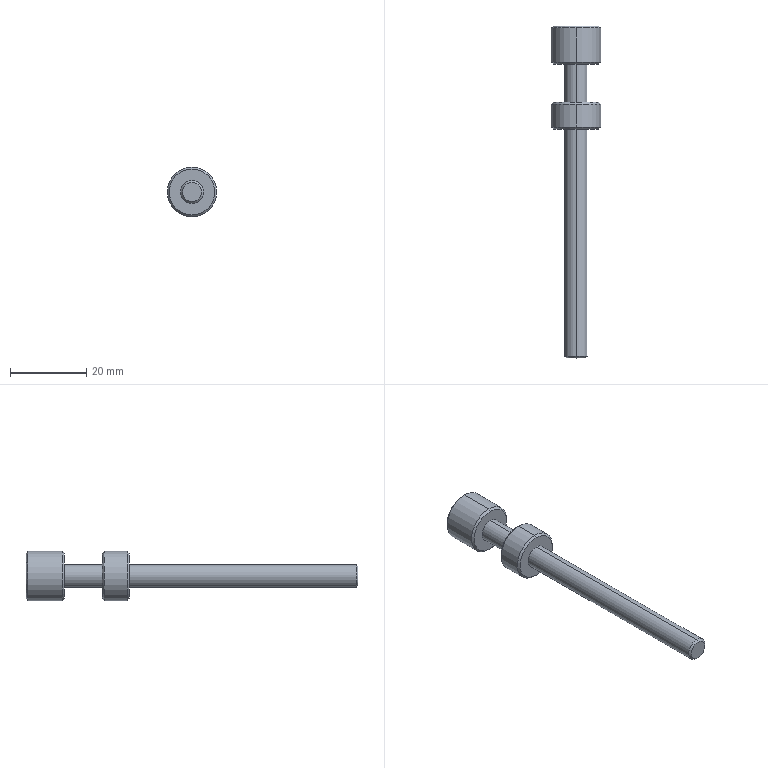Part | SolidWorks | features ICE 5, Chamfer 1, Extrusion 1 | 1 solid | 30 faces | box 13 x 87 x 13 mm | volume 4026 mm3 | plane 12 | cone 10 | cylinder 8 | commonest cylinder face diameters 6 x4 13 x4
STEP:
#1=CARTESIAN_POINT('',(0.,67.,6.));
#2=VERTEX_POINT('',#1);
#3=CARTESIAN_POINT('',(0.,67.,-6.));
#4=VERTEX_POINT('',#3);
#5=CARTESIAN_POINT('',(0.,67.,0.));
#6=DIRECTION('',(0.,1.,0.));
#7=DIRECTION('',(0.,0.,1.));
#8=AXIS2_PLACEMENT_3D('',#5,#6,#7);
#9=CIRCLE('',#8,6.);
#10=EDGE_CURVE('',#2,#4,#9,.T.);
#11=ORIENTED_EDGE('',*,*,#10,.F.);
#12=CARTESIAN_POINT('',(0.,66.5,6.5));
#13=VERTEX_POINT('',#12);
#14=CARTESIAN_POINT('',(0.,67.,6.));
#15=DIRECTION('',(0.,-0.7071,0.7071));
#16=VECTOR('',#15,1000.);
#17=LINE('',#14,#16);
#18=EDGE_CURVE('',#2,#13,#17,.T.);
#19=ORIENTED_EDGE('',*,*,#18,.T.);
#20=CARTESIAN_POINT('',(0.,66.5,-6.5));
#21=VERTEX_POINT('',#20);
#22=CARTESIAN_POINT('',(0.,66.5,0.));
#23=DIRECTION('',(0.,-1.,0.));
#24=DIRECTION('',(0.,0.,1.));
#25=AXIS2_PLACEMENT_3D('',#22,#23,#24);
#26=CIRCLE('',#25,6.5);
#27=EDGE_CURVE('',#21,#13,#26,.T.);
#28=ORIENTED_EDGE('',*,*,#27,.F.);
#29=CARTESIAN_POINT('',(0.,67.,-6.));
#30=DIRECTION('',(0.,-0.7071,-0.7071));
#31=VECTOR('',#30,1000.);
#32=LINE('',#29,#31);
#33=EDGE_CURVE('',#4,#21,#32,.T.);
#34=ORIENTED_EDGE('',*,*,#33,.F.);
#35=EDGE_LOOP('',(#11,#19,#28,#34));
#36=FACE_OUTER_BOUND('',#35,.T.);
#37=CARTESIAN_POINT('',(0.,67.,0.));
#38=DIRECTION('',(0.,-1.,0.));
#39=DIRECTION('',(0.,0.,-1.));
#40=AXIS2_PLACEMENT_3D('',#37,#38,#39);
#41=CONICAL_SURFACE('',#40,6.,0.7854);
#42=ADVANCED_FACE('',(#36),#41,.T.);
#43=CARTESIAN_POINT('',(0.,60.,-6.));
#44=VERTEX_POINT('',#43);
#45=CARTESIAN_POINT('',(0.,60.,6.));
#46=VERTEX_POINT('',#45);
#47=CARTESIAN_POINT('',(0.,60.,0.));
#48=DIRECTION('',(0.,-1.,0.));
#49=DIRECTION('',(0.,0.,1.));
#50=AXIS2_PLACEMENT_3D('',#47,#48,#49);
#51=CIRCLE('',#50,6.);
#52=EDGE_CURVE('',#44,#46,#51,.T.);
#53=ORIENTED_EDGE('',*,*,#52,.F.);
#54=CARTESIAN_POINT('',(0.,60.5,-6.5));
#55=VERTEX_POINT('',#54);
#56=CARTESIAN_POINT('',(0.,60.5,-6.5));
#57=DIRECTION('',(0.,0.7071,-0.7071));
#58=VECTOR('',#57,1000.);
#59=LINE('',#56,#58);
#60=EDGE_CURVE('',#44,#55,#59,.T.);
#61=ORIENTED_EDGE('',*,*,#60,.T.);
#62=CARTESIAN_POINT('',(0.,60.5,6.5));
#63=VERTEX_POINT('',#62);
#64=CARTESIAN_POINT('',(0.,60.5,0.));
#65=DIRECTION('',(0.,1.,0.));
#66=DIRECTION('',(0.,0.,1.));
#67=AXIS2_PLACEMENT_3D('',#64,#65,#66);
#68=CIRCLE('',#67,6.5);
#69=EDGE_CURVE('',#63,#55,#68,.T.);
#70=ORIENTED_EDGE('',*,*,#69,.F.);
#71=CARTESIAN_POINT('',(0.,60.5,6.5));
#72=DIRECTION('',(0.,0.7071,0.7071));
#73=VECTOR('',#72,1000.);
#74=LINE('',#71,#73);
#75=EDGE_CURVE('',#46,#63,#74,.T.);
#76=ORIENTED_EDGE('',*,*,#75,.F.);
#77=EDGE_LOOP('',(#53,#61,#70,#76));
#78=FACE_OUTER_BOUND('',#77,.T.);
#79=CARTESIAN_POINT('',(0.,60.5,0.));
#80=DIRECTION('',(0.,1.,0.));
#81=DIRECTION('',(0.,0.,1.));
#82=AXIS2_PLACEMENT_3D('',#79,#80,#81);
#83=CONICAL_SURFACE('',#82,6.5,0.7854);
#84=ADVANCED_FACE('',(#78),#83,.T.);
#85=CARTESIAN_POINT('',(0.,77.,-6.));
#86=VERTEX_POINT('',#85);
#87=CARTESIAN_POINT('',(0.,77.,6.));
#88=VERTEX_POINT('',#87);
#89=CARTESIAN_POINT('',(0.,77.,0.));
#90=DIRECTION('',(0.,-1.,0.));
#91=DIRECTION('',(0.,0.,1.));
#92=AXIS2_PLACEMENT_3D('',#89,#90,#91);
#93=CIRCLE('',#92,6.);
#94=EDGE_CURVE('',#86,#88,#93,.T.);
#95=ORIENTED_EDGE('',*,*,#94,.F.);
#96=CARTESIAN_POINT('',(0.,77.5,-6.5));
#97=VERTEX_POINT('',#96);
#98=CARTESIAN_POINT('',(0.,77.5,-6.5));
#99=DIRECTION('',(0.,0.7071,-0.7071));
#100=VECTOR('',#99,1000.);
#101=LINE('',#98,#100);
#102=EDGE_CURVE('',#86,#97,#101,.T.);
#103=ORIENTED_EDGE('',*,*,#102,.T.);
#104=CARTESIAN_POINT('',(0.,77.5,6.5));
#105=VERTEX_POINT('',#104);
#106=CARTESIAN_POINT('',(0.,77.5,0.));
#107=DIRECTION('',(0.,1.,0.));
#108=DIRECTION('',(0.,0.,1.));
#109=AXIS2_PLACEMENT_3D('',#106,#107,#108);
#110=CIRCLE('',#109,6.5);
#111=EDGE_CURVE('',#105,#97,#110,.T.);
#112=ORIENTED_EDGE('',*,*,#111,.F.);
#113=CARTESIAN_POINT('',(0.,77.5,6.5));
#114=DIRECTION('',(0.,0.7071,0.7071));
#115=VECTOR('',#114,1000.);
#116=LINE('',#113,#115);
#117=EDGE_CURVE('',#88,#105,#116,.T.);
#118=ORIENTED_EDGE('',*,*,#117,.F.);
#119=EDGE_LOOP('',(#95,#103,#112,#118));
#120=FACE_OUTER_BOUND('',#119,.T.);
#121=CARTESIAN_POINT('',(0.,77.5,0.));
#122=DIRECTION('',(0.,1.,0.));
#123=DIRECTION('',(0.,0.,1.));
#124=AXIS2_PLACEMENT_3D('',#121,#122,#123);
#125=CONICAL_SURFACE('',#124,6.5,0.7854);
#126=ADVANCED_FACE('',(#120),#125,.T.);
#127=CARTESIAN_POINT('',(0.,87.,6.));
#128=VERTEX_POINT('',#127);
#129=CARTESIAN_POINT('',(0.,87.,-6.));
#130=VERTEX_POINT('',#129);
#131=CARTESIAN_POINT('',(0.,87.,0.));
#132=DIRECTION('',(0.,1.,0.));
#133=DIRECTION('',(0.,0.,1.));
#134=AXIS2_PLACEMENT_3D('',#131,#132,#133);
#135=CIRCLE('',#134,6.);
#136=EDGE_CURVE('',#128,#130,#135,.T.);
#137=ORIENTED_EDGE('',*,*,#136,.F.);
#138=CARTESIAN_POINT('',(0.,86.5,6.5));
#139=VERTEX_POINT('',#138);
#140=CARTESIAN_POINT('',(0.,87.,6.));
#141=DIRECTION('',(0.,-0.7071,0.7071));
#142=VECTOR('',#141,1000.);
#143=LINE('',#140,#142);
#144=EDGE_CURVE('',#128,#139,#143,.T.);
#145=ORIENTED_EDGE('',*,*,#144,.T.);
#146=CARTESIAN_POINT('',(0.,86.5,-6.5));
#147=VERTEX_POINT('',#146);
#148=CARTESIAN_POINT('',(0.,86.5,0.));
#149=DIRECTION('',(0.,-1.,0.));
#150=DIRECTION('',(0.,0.,1.));
#151=AXIS2_PLACEMENT_3D('',#148,#149,#150);
#152=CIRCLE('',#151,6.5);
#153=EDGE_CURVE('',#147,#139,#152,.T.);
#154=ORIENTED_EDGE('',*,*,#153,.F.);
#155=CARTESIAN_POINT('',(0.,87.,-6.));
#156=DIRECTION('',(0.,-0.7071,-0.7071));
#157=VECTOR('',#156,1000.);
#158=LINE('',#155,#157);
#159=EDGE_CURVE('',#130,#147,#158,.T.);
#160=ORIENTED_EDGE('',*,*,#159,.F.);
#161=EDGE_LOOP('',(#137,#145,#154,#160));
#162=FACE_OUTER_BOUND('',#161,.T.);
#163=CARTESIAN_POINT('',(0.,87.,0.));
#164=DIRECTION('',(0.,-1.,0.));
#165=DIRECTION('',(0.,0.,-1.));
#166=AXIS2_PLACEMENT_3D('',#163,#164,#165);
#167=CONICAL_SURFACE('',#166,6.,0.7854);
#168=ADVANCED_FACE('',(#162),#167,.T.);
#169=CARTESIAN_POINT('',(0.,0.,-2.5));
#170=VERTEX_POINT('',#169);
#171=CARTESIAN_POINT('',(0.,0.,2.5));
#172=VERTEX_POINT('',#171);
#173=CARTESIAN_POINT('',(0.,0.,0.));
#174=DIRECTION('',(0.,-1.,0.));
#175=DIRECTION('',(0.,0.,1.));
#176=AXIS2_PLACEMENT_3D('',#173,#174,#175);
#177=CIRCLE('',#176,2.5);
#178=EDGE_CURVE('',#170,#172,#177,.T.);
#179=ORIENTED_EDGE('',*,*,#178,.F.);
#180=CARTESIAN_POINT('',(0.,0.5,-3.));
#181=VERTEX_POINT('',#180);
#182=CARTESIAN_POINT('',(0.,0.5,-3.));
#183=DIRECTION('',(0.,0.7071,-0.7071));
#184=VECTOR('',#183,1000.);
#185=LINE('',#182,#184);
#186=EDGE_CURVE('',#170,#181,#185,.T.);
#187=ORIENTED_EDGE('',*,*,#186,.T.);
#188=CARTESIAN_POINT('',(0.,0.5,3.));
#189=VERTEX_POINT('',#188);
#190=CARTESIAN_POINT('',(0.,0.5,0.));
#191=DIRECTION('',(0.,1.,0.));
#192=DIRECTION('',(0.,0.,1.));
#193=AXIS2_PLACEMENT_3D('',#190,#191,#192);
#194=CIRCLE('',#193,3.);
#195=EDGE_CURVE('',#189,#181,#194,.T.);
#196=ORIENTED_EDGE('',*,*,#195,.F.);
#197=CARTESIAN_POINT('',(0.,0.5,3.));
#198=DIRECTION('',(0.,0.7071,0.7071));
#199=VECTOR('',#198,1000.);
#200=LINE('',#197,#199);
#201=EDGE_CURVE('',#172,#189,#200,.T.);
#202=ORIENTED_EDGE('',*,*,#201,.F.);
#203=EDGE_LOOP('',(#179,#187,#196,#202));
#204=FACE_OUTER_BOUND('',#203,.T.);
#205=CARTESIAN_POINT('',(0.,0.5,0.));
#206=DIRECTION('',(0.,1.,0.));
#207=DIRECTION('',(0.,0.,1.));
#208=AXIS2_PLACEMENT_3D('',#205,#206,#207);
#209=CONICAL_SURFACE('',#208,3.,0.7854);
#210=ADVANCED_FACE('',(#204),#209,.T.);
#211=ORIENTED_EDGE('',*,*,#153,.T.);
#212=CARTESIAN_POINT('',(0.,87.,6.5));
#213=DIRECTION('',(0.,-1.,0.));
#214=VECTOR('',#213,1000.);
#215=LINE('',#212,#214);
#216=EDGE_CURVE('',#139,#105,#215,.T.);
#217=ORIENTED_EDGE('',*,*,#216,.T.);
#218=ORIENTED_EDGE('',*,*,#111,.T.);
#219=CARTESIAN_POINT('',(0.,87.,-6.5));
#220=DIRECTION('',(0.,-1.,0.));
#221=VECTOR('',#220,1000.);
#222=LINE('',#219,#221);
#223=EDGE_CURVE('',#147,#97,#222,.T.);
#224=ORIENTED_EDGE('',*,*,#223,.F.);
#225=EDGE_LOOP('',(#211,#217,#218,#224));
#226=FACE_OUTER_BOUND('',#225,.T.);
#227=CARTESIAN_POINT('',(0.,87.,0.));
#228=DIRECTION('',(0.,-1.,0.));
#229=DIRECTION('',(0.,0.,-1.));
#230=AXIS2_PLACEMENT_3D('',#227,#228,#229);
#231=CYLINDRICAL_SURFACE('',#230,6.5);
#232=ADVANCED_FACE('',(#226),#231,.T.);
#233=CARTESIAN_POINT('',(0.,77.,3.));
#234=VERTEX_POINT('',#233);
#235=CARTESIAN_POINT('',(0.,77.,-3.));
#236=VERTEX_POINT('',#235);
#237=CARTESIAN_POINT('',(0.,77.,0.));
#238=DIRECTION('',(0.,1.,0.));
#239=DIRECTION('',(0.,0.,1.));
#240=AXIS2_PLACEMENT_3D('',#237,#238,#239);
#241=CIRCLE('',#240,3.);
#242=EDGE_CURVE('',#234,#236,#241,.T.);
#243=ORIENTED_EDGE('',*,*,#242,.F.);
#244=CARTESIAN_POINT('',(0.,67.,3.));
#245=VERTEX_POINT('',#244);
#246=CARTESIAN_POINT('',(0.,77.,3.));
#247=DIRECTION('',(0.,-1.,0.));
#248=VECTOR('',#247,1000.);
#249=LINE('',#246,#248);
#250=EDGE_CURVE('',#234,#245,#249,.T.);
#251=ORIENTED_EDGE('',*,*,#250,.T.);
#252=CARTESIAN_POINT('',(0.,67.,-3.));
#253=VERTEX_POINT('',#252);
#254=CARTESIAN_POINT('',(0.,67.,0.));
#255=DIRECTION('',(0.,1.,0.));
#256=DIRECTION('',(0.,0.,1.));
#257=AXIS2_PLACEMENT_3D('',#254,#255,#256);
#258=CIRCLE('',#257,3.);
#259=EDGE_CURVE('',#245,#253,#258,.T.);
#260=ORIENTED_EDGE('',*,*,#259,.T.);
#261=CARTESIAN_POINT('',(0.,77.,-3.));
#262=DIRECTION('',(0.,-1.,0.));
#263=VECTOR('',#262,1000.);
#264=LINE('',#261,#263);
#265=EDGE_CURVE('',#236,#253,#264,.T.);
#266=ORIENTED_EDGE('',*,*,#265,.F.);
#267=EDGE_LOOP('',(#243,#251,#260,#266));
#268=FACE_OUTER_BOUND('',#267,.T.);
#269=CARTESIAN_POINT('',(0.,77.,0.));
#270=DIRECTION('',(0.,-1.,0.));
#271=DIRECTION('',(0.,0.,-1.));
#272=AXIS2_PLACEMENT_3D('',#269,#270,#271);
#273=CYLINDRICAL_SURFACE('',#272,3.);
#274=ADVANCED_FACE('',(#268),#273,.T.);
#275=ORIENTED_EDGE('',*,*,#27,.T.);
#276=CARTESIAN_POINT('',(0.,67.,6.5));
#277=DIRECTION('',(0.,-1.,0.));
#278=VECTOR('',#277,1000.);
#279=LINE('',#276,#278);
#280=EDGE_CURVE('',#13,#63,#279,.T.);
#281=ORIENTED_EDGE('',*,*,#280,.T.);
#282=ORIENTED_EDGE('',*,*,#69,.T.);
#283=CARTESIAN_POINT('',(0.,67.,-6.5));
#284=DIRECTION('',(0.,-1.,0.));
#285=VECTOR('',#284,1000.);
#286=LINE('',#283,#285);
#287=EDGE_CURVE('',#21,#55,#286,.T.);
#288=ORIENTED_EDGE('',*,*,#287,.F.);
#289=EDGE_LOOP('',(#275,#281,#282,#288));
#290=FACE_OUTER_BOUND('',#289,.T.);
#291=CARTESIAN_POINT('',(0.,67.,0.));
#292=DIRECTION('',(0.,-1.,0.));
#293=DIRECTION('',(0.,0.,-1.));
#294=AXIS2_PLACEMENT_3D('',#291,#292,#293);
#295=CYLINDRICAL_SURFACE('',#294,6.5);
#296=ADVANCED_FACE('',(#290),#295,.T.);
#297=CARTESIAN_POINT('',(0.,60.,3.));
#298=VERTEX_POINT('',#297);
#299=CARTESIAN_POINT('',(0.,60.,-3.));
#300=VERTEX_POINT('',#299);
#301=CARTESIAN_POINT('',(0.,60.,0.));
#302=DIRECTION('',(0.,1.,0.));
#303=DIRECTION('',(0.,0.,1.));
#304=AXIS2_PLACEMENT_3D('',#301,#302,#303);
#305=CIRCLE('',#304,3.);
#306=EDGE_CURVE('',#298,#300,#305,.T.);
#307=ORIENTED_EDGE('',*,*,#306,.F.);
#308=CARTESIAN_POINT('',(0.,45.,3.));
#309=DIRECTION('',(0.,-1.,0.));
#310=VECTOR('',#309,1000.);
#311=LINE('',#308,#310);
#312=EDGE_CURVE('',#298,#189,#311,.T.);
#313=ORIENTED_EDGE('',*,*,#312,.T.);
#314=ORIENTED_EDGE('',*,*,#195,.T.);
#315=CARTESIAN_POINT('',(0.,45.,-3.));
#316=DIRECTION('',(0.,-1.,0.));
#317=VECTOR('',#316,1000.);
#318=LINE('',#315,#317);
#319=EDGE_CURVE('',#300,#181,#318,.T.);
#320=ORIENTED_EDGE('',*,*,#319,.F.);
#321=EDGE_LOOP('',(#307,#313,#314,#320));
#322=FACE_OUTER_BOUND('',#321,.T.);
#323=CARTESIAN_POINT('',(0.,45.,0.));
#324=DIRECTION('',(0.,-1.,0.));
#325=DIRECTION('',(0.,0.,-1.));
#326=AXIS2_PLACEMENT_3D('',#323,#324,#325);
#327=CYLINDRICAL_SURFACE('',#326,3.);
#328=ADVANCED_FACE('',(#322),#327,.T.);
#329=CARTESIAN_POINT('',(0.,67.,0.));
#330=DIRECTION('',(0.,1.,0.));
#331=DIRECTION('',(0.,0.,1.));
#332=AXIS2_PLACEMENT_3D('',#329,#330,#331);
#333=CIRCLE('',#332,6.);
#334=EDGE_CURVE('',#4,#2,#333,.T.);
#335=ORIENTED_EDGE('',*,*,#334,.T.);
#336=ORIENTED_EDGE('',*,*,#10,.T.);
#337=EDGE_LOOP('',(#335,#336));
#338=FACE_OUTER_BOUND('',#337,.T.);
#339=CARTESIAN_POINT('',(0.,67.,0.));
#340=DIRECTION('',(0.,1.,0.));
#341=DIRECTION('',(0.,0.,1.));
#342=AXIS2_PLACEMENT_3D('',#339,#340,#341);
#343=CIRCLE('',#342,3.);
#344=EDGE_CURVE('',#253,#245,#343,.T.);
#345=ORIENTED_EDGE('',*,*,#344,.F.);
#346=ORIENTED_EDGE('',*,*,#259,.F.);
#347=EDGE_LOOP('',(#345,#346));
#348=FACE_BOUND('',#347,.T.);
#349=CARTESIAN_POINT('',(0.,67.,0.));
#350=DIRECTION('',(0.,1.,0.));
#351=DIRECTION('',(0.,0.,1.));
#352=AXIS2_PLACEMENT_3D('',#349,#350,#351);
#353=PLANE('',#352);
#354=ADVANCED_FACE('',(#338,#348),#353,.T.);
#355=ORIENTED_EDGE('',*,*,#312,.F.);
#356=CARTESIAN_POINT('',(0.,60.,0.));
#357=DIRECTION('',(0.,1.,0.));
#358=DIRECTION('',(0.,0.,1.));
#359=AXIS2_PLACEMENT_3D('',#356,#357,#358);
#360=CIRCLE('',#359,3.);
#361=EDGE_CURVE('',#300,#298,#360,.T.);
#362=ORIENTED_EDGE('',*,*,#361,.F.);
#363=ORIENTED_EDGE('',*,*,#319,.T.);
#364=CARTESIAN_POINT('',(0.,0.5,0.));
#365=DIRECTION('',(0.,1.,0.));
#366=DIRECTION('',(0.,0.,1.));
#367=AXIS2_PLACEMENT_3D('',#364,#365,#366);
#368=CIRCLE('',#367,3.);
#369=EDGE_CURVE('',#181,#189,#368,.T.);
#370=ORIENTED_EDGE('',*,*,#369,.T.);
#371=EDGE_LOOP('',(#355,#362,#363,#370));
#372=FACE_OUTER_BOUND('',#371,.T.);
#373=CARTESIAN_POINT('',(0.,45.,0.));
#374=DIRECTION('',(0.,-1.,0.));
#375=DIRECTION('',(0.,0.,-1.));
#376=AXIS2_PLACEMENT_3D('',#373,#374,#375);
#377=CYLINDRICAL_SURFACE('',#376,3.);
#378=ADVANCED_FACE('',(#372),#377,.T.);
#379=CARTESIAN_POINT('',(0.,0.,0.));
#380=DIRECTION('',(0.,-1.,0.));
#381=DIRECTION('',(0.,0.,1.));
#382=AXIS2_PLACEMENT_3D('',#379,#380,#381);
#383=CIRCLE('',#382,2.5);
#384=EDGE_CURVE('',#172,#170,#383,.T.);
#385=ORIENTED_EDGE('',*,*,#384,.T.);
#386=ORIENTED_EDGE('',*,*,#178,.T.);
#387=EDGE_LOOP('',(#385,#386));
#388=FACE_OUTER_BOUND('',#387,.T.);
#389=CARTESIAN_POINT('',(0.,0.,0.));
#390=DIRECTION('',(0.,1.,0.));
#391=DIRECTION('',(0.,0.,1.));
#392=AXIS2_PLACEMENT_3D('',#389,#390,#391);
#393=PLANE('',#392);
#394=ADVANCED_FACE('',(#388),#393,.F.);
#395=CARTESIAN_POINT('',(0.,60.,0.));
#396=DIRECTION('',(0.,-1.,0.));
#397=DIRECTION('',(0.,0.,1.));
#398=AXIS2_PLACEMENT_3D('',#395,#396,#397);
#399=CIRCLE('',#398,6.);
#400=EDGE_CURVE('',#46,#44,#399,.T.);
#401=ORIENTED_EDGE('',*,*,#400,.T.);
#402=ORIENTED_EDGE('',*,*,#52,.T.);
#403=EDGE_LOOP('',(#401,#402));
#404=FACE_OUTER_BOUND('',#403,.T.);
#405=ORIENTED_EDGE('',*,*,#361,.T.);
#406=ORIENTED_EDGE('',*,*,#306,.T.);
#407=EDGE_LOOP('',(#405,#406));
#408=FACE_BOUND('',#407,.T.);
#409=CARTESIAN_POINT('',(0.,60.,0.));
#410=DIRECTION('',(0.,1.,0.));
#411=DIRECTION('',(0.,0.,1.));
#412=AXIS2_PLACEMENT_3D('',#409,#410,#411);
#413=PLANE('',#412);
#414=ADVANCED_FACE('',(#404,#408),#413,.F.);
#415=ORIENTED_EDGE('',*,*,#280,.F.);
#416=CARTESIAN_POINT('',(0.,66.5,0.));
#417=DIRECTION('',(0.,-1.,0.));
#418=DIRECTION('',(0.,0.,1.));
#419=AXIS2_PLACEMENT_3D('',#416,#417,#418);
#420=CIRCLE('',#419,6.5);
#421=EDGE_CURVE('',#13,#21,#420,.T.);
#422=ORIENTED_EDGE('',*,*,#421,.T.);
#423=ORIENTED_EDGE('',*,*,#287,.T.);
#424=CARTESIAN_POINT('',(0.,60.5,0.));
#425=DIRECTION('',(0.,1.,0.));
#426=DIRECTION('',(0.,0.,1.));
#427=AXIS2_PLACEMENT_3D('',#424,#425,#426);
#428=CIRCLE('',#427,6.5);
#429=EDGE_CURVE('',#55,#63,#428,.T.);
#430=ORIENTED_EDGE('',*,*,#429,.T.);
#431=EDGE_LOOP('',(#415,#422,#423,#430));
#432=FACE_OUTER_BOUND('',#431,.T.);
#433=CARTESIAN_POINT('',(0.,67.,0.));
#434=DIRECTION('',(0.,-1.,0.));
#435=DIRECTION('',(0.,0.,-1.));
#436=AXIS2_PLACEMENT_3D('',#433,#434,#435);
#437=CYLINDRICAL_SURFACE('',#436,6.5);
#438=ADVANCED_FACE('',(#432),#437,.T.);
#439=ORIENTED_EDGE('',*,*,#250,.F.);
#440=CARTESIAN_POINT('',(0.,77.,0.));
#441=DIRECTION('',(0.,1.,0.));
#442=DIRECTION('',(0.,0.,1.));
#443=AXIS2_PLACEMENT_3D('',#440,#441,#442);
#444=CIRCLE('',#443,3.);
#445=EDGE_CURVE('',#236,#234,#444,.T.);
#446=ORIENTED_EDGE('',*,*,#445,.F.);
#447=ORIENTED_EDGE('',*,*,#265,.T.);
#448=ORIENTED_EDGE('',*,*,#344,.T.);
#449=EDGE_LOOP('',(#439,#446,#447,#448));
#450=FACE_OUTER_BOUND('',#449,.T.);
#451=CARTESIAN_POINT('',(0.,77.,0.));
#452=DIRECTION('',(0.,-1.,0.));
#453=DIRECTION('',(0.,0.,-1.));
#454=AXIS2_PLACEMENT_3D('',#451,#452,#453);
#455=CYLINDRICAL_SURFACE('',#454,3.);
#456=ADVANCED_FACE('',(#450),#455,.T.);
#457=CARTESIAN_POINT('',(0.,77.,0.));
#458=DIRECTION('',(0.,-1.,0.));
#459=DIRECTION('',(0.,0.,1.));
#460=AXIS2_PLACEMENT_3D('',#457,#458,#459);
#461=CIRCLE('',#460,6.);
#462=EDGE_CURVE('',#88,#86,#461,.T.);
#463=ORIENTED_EDGE('',*,*,#462,.T.);
#464=ORIENTED_EDGE('',*,*,#94,.T.);
#465=EDGE_LOOP('',(#463,#464));
#466=FACE_OUTER_BOUND('',#465,.T.);
#467=ORIENTED_EDGE('',*,*,#445,.T.);
#468=ORIENTED_EDGE('',*,*,#242,.T.);
#469=EDGE_LOOP('',(#467,#468));
#470=FACE_BOUND('',#469,.T.);
#471=CARTESIAN_POINT('',(0.,77.,0.));
#472=DIRECTION('',(0.,1.,0.));
#473=DIRECTION('',(0.,0.,1.));
#474=AXIS2_PLACEMENT_3D('',#471,#472,#473);
#475=PLANE('',#474);
#476=ADVANCED_FACE('',(#466,#470),#475,.F.);
#477=ORIENTED_EDGE('',*,*,#216,.F.);
#478=CARTESIAN_POINT('',(0.,86.5,0.));
#479=DIRECTION('',(0.,-1.,0.));
#480=DIRECTION('',(0.,0.,1.));
#481=AXIS2_PLACEMENT_3D('',#478,#479,#480);
#482=CIRCLE('',#481,6.5);
#483=EDGE_CURVE('',#139,#147,#482,.T.);
#484=ORIENTED_EDGE('',*,*,#483,.T.);
#485=ORIENTED_EDGE('',*,*,#223,.T.);
#486=CARTESIAN_POINT('',(0.,77.5,0.));
#487=DIRECTION('',(0.,1.,0.));
#488=DIRECTION('',(0.,0.,1.));
#489=AXIS2_PLACEMENT_3D('',#486,#487,#488);
#490=CIRCLE('',#489,6.5);
#491=EDGE_CURVE('',#97,#105,#490,.T.);
#492=ORIENTED_EDGE('',*,*,#491,.T.);
#493=EDGE_LOOP('',(#477,#484,#485,#492));
#494=FACE_OUTER_BOUND('',#493,.T.);
#495=CARTESIAN_POINT('',(0.,87.,0.));
#496=DIRECTION('',(0.,-1.,0.));
#497=DIRECTION('',(0.,0.,-1.));
#498=AXIS2_PLACEMENT_3D('',#495,#496,#497);
#499=CYLINDRICAL_SURFACE('',#498,6.5);
#500=ADVANCED_FACE('',(#494),#499,.T.);
#501=CARTESIAN_POINT('',(0.,87.,0.));
#502=DIRECTION('',(0.,1.,0.));
#503=DIRECTION('',(0.,0.,1.));
#504=AXIS2_PLACEMENT_3D('',#501,#502,#503);
#505=CIRCLE('',#504,6.);
#506=EDGE_CURVE('',#130,#128,#505,.T.);
#507=ORIENTED_EDGE('',*,*,#506,.T.);
#508=ORIENTED_EDGE('',*,*,#136,.T.);
#509=EDGE_LOOP('',(#507,#508));
#510=FACE_OUTER_BOUND('',#509,.T.);
#511=CARTESIAN_POINT('',(3.,87.,-1.732));
#512=VERTEX_POINT('',#511);
#513=CARTESIAN_POINT('',(0.,87.,-3.464));
#514=VERTEX_POINT('',#513);
#515=CARTESIAN_POINT('',(3.,87.,-1.732));
#516=DIRECTION('',(-0.866,0.,-0.5));
#517=VECTOR('',#516,1000.);
#518=LINE('',#515,#517);
#519=EDGE_CURVE('',#512,#514,#518,.T.);
#520=ORIENTED_EDGE('',*,*,#519,.F.);
#521=CARTESIAN_POINT('',(3.,87.,1.732));
#522=VERTEX_POINT('',#521);
#523=CARTESIAN_POINT('',(3.,87.,1.732));
#524=DIRECTION('',(0.,0.,-1.));
#525=VECTOR('',#524,1000.);
#526=LINE('',#523,#525);
#527=EDGE_CURVE('',#522,#512,#526,.T.);
#528=ORIENTED_EDGE('',*,*,#527,.F.);
#529=CARTESIAN_POINT('',(0.,87.,3.464));
#530=VERTEX_POINT('',#529);
#531=CARTESIAN_POINT('',(0.,87.,3.464));
#532=DIRECTION('',(0.866,0.,-0.5));
#533=VECTOR('',#532,1000.);
#534=LINE('',#531,#533);
#535=EDGE_CURVE('',#530,#522,#534,.T.);
#536=ORIENTED_EDGE('',*,*,#535,.F.);
#537=CARTESIAN_POINT('',(-3.,87.,1.732));
#538=VERTEX_POINT('',#537);
#539=CARTESIAN_POINT('',(-3.,87.,1.732));
#540=DIRECTION('',(0.866,0.,0.5));
#541=VECTOR('',#540,1000.);
#542=LINE('',#539,#541);
#543=EDGE_CURVE('',#538,#530,#542,.T.);
#544=ORIENTED_EDGE('',*,*,#543,.F.);
#545=CARTESIAN_POINT('',(-3.,87.,-1.732));
#546=VERTEX_POINT('',#545);
#547=CARTESIAN_POINT('',(-3.,87.,-1.732));
#548=DIRECTION('',(0.,0.,1.));
#549=VECTOR('',#548,1000.);
#550=LINE('',#547,#549);
#551=EDGE_CURVE('',#546,#538,#550,.T.);
#552=ORIENTED_EDGE('',*,*,#551,.F.);
#553=CARTESIAN_POINT('',(0.,87.,-3.464));
#554=DIRECTION('',(-0.866,0.,0.5));
#555=VECTOR('',#554,1000.);
#556=LINE('',#553,#555);
#557=EDGE_CURVE('',#514,#546,#556,.T.);
#558=ORIENTED_EDGE('',*,*,#557,.F.);
#559=EDGE_LOOP('',(#520,#528,#536,#544,#552,#558));
#560=FACE_BOUND('',#559,.T.);
#561=CARTESIAN_POINT('',(0.,87.,0.));
#562=DIRECTION('',(0.,1.,0.));
#563=DIRECTION('',(0.,0.,1.));
#564=AXIS2_PLACEMENT_3D('',#561,#562,#563);
#565=PLANE('',#564);
#566=ADVANCED_FACE('',(#510,#560),#565,.T.);
#567=ORIENTED_EDGE('',*,*,#519,.T.);
#568=CARTESIAN_POINT('',(0.,81.,-3.464));
#569=VERTEX_POINT('',#568);
#570=CARTESIAN_POINT('',(0.,81.,-3.464));
#571=DIRECTION('',(0.,1.,0.));
#572=VECTOR('',#571,1000.);
#573=LINE('',#570,#572);
#574=EDGE_CURVE('',#569,#514,#573,.T.);
#575=ORIENTED_EDGE('',*,*,#574,.F.);
#576=CARTESIAN_POINT('',(3.,81.,-1.732));
#577=VERTEX_POINT('',#576);
#578=CARTESIAN_POINT('',(3.,81.,-1.732));
#579=DIRECTION('',(-0.866,0.,-0.5));
#580=VECTOR('',#579,1000.);
#581=LINE('',#578,#580);
#582=EDGE_CURVE('',#577,#569,#581,.T.);
#583=ORIENTED_EDGE('',*,*,#582,.F.);
#584=CARTESIAN_POINT('',(3.,81.,-1.732));
#585=DIRECTION('',(0.,1.,0.));
#586=VECTOR('',#585,1000.);
#587=LINE('',#584,#586);
#588=EDGE_CURVE('',#577,#512,#587,.T.);
#589=ORIENTED_EDGE('',*,*,#588,.T.);
#590=EDGE_LOOP('',(#567,#575,#583,#589));
#591=FACE_OUTER_BOUND('',#590,.T.);
#592=CARTESIAN_POINT('',(3.,81.,-1.732));
#593=DIRECTION('',(0.5,0.,-0.866));
#594=DIRECTION('',(-0.866,0.,-0.5));
#595=AXIS2_PLACEMENT_3D('',#592,#593,#594);
#596=PLANE('',#595);
#597=ADVANCED_FACE('',(#591),#596,.F.);
#598=ORIENTED_EDGE('',*,*,#527,.T.);
#599=ORIENTED_EDGE('',*,*,#588,.F.);
#600=CARTESIAN_POINT('',(3.,81.,1.732));
#601=VERTEX_POINT('',#600);
#602=CARTESIAN_POINT('',(3.,81.,1.732));
#603=DIRECTION('',(0.,0.,-1.));
#604=VECTOR('',#603,1000.);
#605=LINE('',#602,#604);
#606=EDGE_CURVE('',#601,#577,#605,.T.);
#607=ORIENTED_EDGE('',*,*,#606,.F.);
#608=CARTESIAN_POINT('',(3.,81.,1.732));
#609=DIRECTION('',(0.,1.,0.));
#610=VECTOR('',#609,1000.);
#611=LINE('',#608,#610);
#612=EDGE_CURVE('',#601,#522,#611,.T.);
#613=ORIENTED_EDGE('',*,*,#612,.T.);
#614=EDGE_LOOP('',(#598,#599,#607,#613));
#615=FACE_OUTER_BOUND('',#614,.T.);
#616=CARTESIAN_POINT('',(3.,81.,1.732));
#617=DIRECTION('',(1.,0.,0.));
#618=DIRECTION('',(0.,0.,-1.));
#619=AXIS2_PLACEMENT_3D('',#616,#617,#618);
#620=PLANE('',#619);
#621=ADVANCED_FACE('',(#615),#620,.F.);
#622=ORIENTED_EDGE('',*,*,#535,.T.);
#623=ORIENTED_EDGE('',*,*,#612,.F.);
#624=CARTESIAN_POINT('',(0.,81.,3.464));
#625=VERTEX_POINT('',#624);
#626=CARTESIAN_POINT('',(0.,81.,3.464));
#627=DIRECTION('',(0.866,0.,-0.5));
#628=VECTOR('',#627,1000.);
#629=LINE('',#626,#628);
#630=EDGE_CURVE('',#625,#601,#629,.T.);
#631=ORIENTED_EDGE('',*,*,#630,.F.);
#632=CARTESIAN_POINT('',(0.,81.,3.464));
#633=DIRECTION('',(0.,1.,0.));
#634=VECTOR('',#633,1000.);
#635=LINE('',#632,#634);
#636=EDGE_CURVE('',#625,#530,#635,.T.);
#637=ORIENTED_EDGE('',*,*,#636,.T.);
#638=EDGE_LOOP('',(#622,#623,#631,#637));
#639=FACE_OUTER_BOUND('',#638,.T.);
#640=CARTESIAN_POINT('',(0.,81.,3.464));
#641=DIRECTION('',(0.5,0.,0.866));
#642=DIRECTION('',(0.866,0.,-0.5));
#643=AXIS2_PLACEMENT_3D('',#640,#641,#642);
#644=PLANE('',#643);
#645=ADVANCED_FACE('',(#639),#644,.F.);
#646=ORIENTED_EDGE('',*,*,#543,.T.);
#647=ORIENTED_EDGE('',*,*,#636,.F.);
#648=CARTESIAN_POINT('',(-3.,81.,1.732));
#649=VERTEX_POINT('',#648);
#650=CARTESIAN_POINT('',(-3.,81.,1.732));
#651=DIRECTION('',(0.866,0.,0.5));
#652=VECTOR('',#651,1000.);
#653=LINE('',#650,#652);
#654=EDGE_CURVE('',#649,#625,#653,.T.);
#655=ORIENTED_EDGE('',*,*,#654,.F.);
#656=CARTESIAN_POINT('',(-3.,81.,1.732));
#657=DIRECTION('',(0.,1.,0.));
#658=VECTOR('',#657,1000.);
#659=LINE('',#656,#658);
#660=EDGE_CURVE('',#649,#538,#659,.T.);
#661=ORIENTED_EDGE('',*,*,#660,.T.);
#662=EDGE_LOOP('',(#646,#647,#655,#661));
#663=FACE_OUTER_BOUND('',#662,.T.);
#664=CARTESIAN_POINT('',(-3.,81.,1.732));
#665=DIRECTION('',(-0.5,0.,0.866));
#666=DIRECTION('',(0.866,0.,0.5));
#667=AXIS2_PLACEMENT_3D('',#664,#665,#666);
#668=PLANE('',#667);
#669=ADVANCED_FACE('',(#663),#668,.F.);
#670=ORIENTED_EDGE('',*,*,#551,.T.);
#671=ORIENTED_EDGE('',*,*,#660,.F.);
#672=CARTESIAN_POINT('',(-3.,81.,-1.732));
#673=VERTEX_POINT('',#672);
#674=CARTESIAN_POINT('',(-3.,81.,-1.732));
#675=DIRECTION('',(0.,0.,1.));
#676=VECTOR('',#675,1000.);
#677=LINE('',#674,#676);
#678=EDGE_CURVE('',#673,#649,#677,.T.);
#679=ORIENTED_EDGE('',*,*,#678,.F.);
#680=CARTESIAN_POINT('',(-3.,81.,-1.732));
#681=DIRECTION('',(0.,1.,0.));
#682=VECTOR('',#681,1000.);
#683=LINE('',#680,#682);
#684=EDGE_CURVE('',#673,#546,#683,.T.);
#685=ORIENTED_EDGE('',*,*,#684,.T.);
#686=EDGE_LOOP('',(#670,#671,#679,#685));
#687=FACE_OUTER_BOUND('',#686,.T.);
#688=CARTESIAN_POINT('',(-3.,81.,-1.732));
#689=DIRECTION('',(-1.,0.,0.));
#690=DIRECTION('',(0.,0.,1.));
#691=AXIS2_PLACEMENT_3D('',#688,#689,#690);
#692=PLANE('',#691);
#693=ADVANCED_FACE('',(#687),#692,.F.);
#694=ORIENTED_EDGE('',*,*,#557,.T.);
#695=ORIENTED_EDGE('',*,*,#684,.F.);
#696=CARTESIAN_POINT('',(0.,81.,-3.464));
#697=DIRECTION('',(-0.866,0.,0.5));
#698=VECTOR('',#697,1000.);
#699=LINE('',#696,#698);
#700=EDGE_CURVE('',#569,#673,#699,.T.);
#701=ORIENTED_EDGE('',*,*,#700,.F.);
#702=ORIENTED_EDGE('',*,*,#574,.T.);
#703=EDGE_LOOP('',(#694,#695,#701,#702));
#704=FACE_OUTER_BOUND('',#703,.T.);
#705=CARTESIAN_POINT('',(0.,81.,-3.464));
#706=DIRECTION('',(-0.5,0.,-0.866));
#707=DIRECTION('',(-0.866,0.,0.5));
#708=AXIS2_PLACEMENT_3D('',#705,#706,#707);
#709=PLANE('',#708);
#710=ADVANCED_FACE('',(#704),#709,.F.);
#711=ORIENTED_EDGE('',*,*,#582,.T.);
#712=ORIENTED_EDGE('',*,*,#700,.T.);
#713=ORIENTED_EDGE('',*,*,#678,.T.);
#714=ORIENTED_EDGE('',*,*,#654,.T.);
#715=ORIENTED_EDGE('',*,*,#630,.T.);
#716=ORIENTED_EDGE('',*,*,#606,.T.);
#717=EDGE_LOOP('',(#711,#712,#713,#714,#715,#716));
#718=FACE_OUTER_BOUND('',#717,.T.);
#719=CARTESIAN_POINT('',(0.,81.,0.));
#720=DIRECTION('',(0.,1.,0.));
#721=DIRECTION('',(0.,0.,1.));
#722=AXIS2_PLACEMENT_3D('',#719,#720,#721);
#723=PLANE('',#722);
#724=ADVANCED_FACE('',(#718),#723,.T.);
#725=ORIENTED_EDGE('',*,*,#186,.F.);
#726=ORIENTED_EDGE('',*,*,#384,.F.);
#727=ORIENTED_EDGE('',*,*,#201,.T.);
#728=ORIENTED_EDGE('',*,*,#369,.F.);
#729=EDGE_LOOP('',(#725,#726,#727,#728));
#730=FACE_OUTER_BOUND('',#729,.T.);
#731=CARTESIAN_POINT('',(0.,0.5,0.));
#732=DIRECTION('',(0.,1.,0.));
#733=DIRECTION('',(0.,0.,1.));
#734=AXIS2_PLACEMENT_3D('',#731,#732,#733);
#735=CONICAL_SURFACE('',#734,3.,0.7854);
#736=ADVANCED_FACE('',(#730),#735,.T.);
#737=ORIENTED_EDGE('',*,*,#144,.F.);
#738=ORIENTED_EDGE('',*,*,#506,.F.);
#739=ORIENTED_EDGE('',*,*,#159,.T.);
#740=ORIENTED_EDGE('',*,*,#483,.F.);
#741=EDGE_LOOP('',(#737,#738,#739,#740));
#742=FACE_OUTER_BOUND('',#741,.T.);
#743=CARTESIAN_POINT('',(0.,87.,0.));
#744=DIRECTION('',(0.,-1.,0.));
#745=DIRECTION('',(0.,0.,-1.));
#746=AXIS2_PLACEMENT_3D('',#743,#744,#745);
#747=CONICAL_SURFACE('',#746,6.,0.7854);
#748=ADVANCED_FACE('',(#742),#747,.T.);
#749=ORIENTED_EDGE('',*,*,#102,.F.);
#750=ORIENTED_EDGE('',*,*,#462,.F.);
#751=ORIENTED_EDGE('',*,*,#117,.T.);
#752=ORIENTED_EDGE('',*,*,#491,.F.);
#753=EDGE_LOOP('',(#749,#750,#751,#752));
#754=FACE_OUTER_BOUND('',#753,.T.);
#755=CARTESIAN_POINT('',(0.,77.5,0.));
#756=DIRECTION('',(0.,1.,0.));
#757=DIRECTION('',(0.,0.,1.));
#758=AXIS2_PLACEMENT_3D('',#755,#756,#757);
#759=CONICAL_SURFACE('',#758,6.5,0.7854);
#760=ADVANCED_FACE('',(#754),#759,.T.);
#761=ORIENTED_EDGE('',*,*,#60,.F.);
#762=ORIENTED_EDGE('',*,*,#400,.F.);
#763=ORIENTED_EDGE('',*,*,#75,.T.);
#764=ORIENTED_EDGE('',*,*,#429,.F.);
#765=EDGE_LOOP('',(#761,#762,#763,#764));
#766=FACE_OUTER_BOUND('',#765,.T.);
#767=CARTESIAN_POINT('',(0.,60.5,0.));
#768=DIRECTION('',(0.,1.,0.));
#769=DIRECTION('',(0.,0.,1.));
#770=AXIS2_PLACEMENT_3D('',#767,#768,#769);
#771=CONICAL_SURFACE('',#770,6.5,0.7854);
#772=ADVANCED_FACE('',(#766),#771,.T.);
#773=ORIENTED_EDGE('',*,*,#18,.F.);
#774=ORIENTED_EDGE('',*,*,#334,.F.);
#775=ORIENTED_EDGE('',*,*,#33,.T.);
#776=ORIENTED_EDGE('',*,*,#421,.F.);
#777=EDGE_LOOP('',(#773,#774,#775,#776));
#778=FACE_OUTER_BOUND('',#777,.T.);
#779=CARTESIAN_POINT('',(0.,67.,0.));
#780=DIRECTION('',(0.,-1.,0.));
#781=DIRECTION('',(0.,0.,-1.));
#782=AXIS2_PLACEMENT_3D('',#779,#780,#781);
#783=CONICAL_SURFACE('',#782,6.,0.7854);
#784=ADVANCED_FACE('',(#778),#783,.T.);
#785=CLOSED_SHELL('',(#42,#84,#126,#168,#210,#232,#274,#296,#328,#354,#378,#394,#414,#438,#456,#476,#500,#566,#597,#621,#645,#669,#693,#710,#724,#736,#748,#760,#772,#784));
#786=MANIFOLD_SOLID_BREP('',#785);
#787=CARTESIAN_POINT('',(0.,0.,0.));
#788=DIRECTION('',(0.,0.,1.));
#789=DIRECTION('',(1.,0.,0.));
#790=AXIS2_PLACEMENT_3D('',#787,#788,#789);
#791=(LENGTH_UNIT()NAMED_UNIT(*)SI_UNIT(.MILLI.,.METRE.));
#792=UNCERTAINTY_MEASURE_WITH_UNIT(LENGTH_MEASURE(0.00001),#791,'','');
#793=(NAMED_UNIT(*)PLANE_ANGLE_UNIT()SI_UNIT($,.RADIAN.));
#794=(NAMED_UNIT(*)SI_UNIT($,.STERADIAN.)SOLID_ANGLE_UNIT());
#795=(GEOMETRIC_REPRESENTATION_CONTEXT(3)GLOBAL_UNCERTAINTY_ASSIGNED_CONTEXT((#792))GLOBAL_UNIT_ASSIGNED_CONTEXT((#791,#793,#794))REPRESENTATION_CONTEXT('',''));
#796=ADVANCED_BREP_SHAPE_REPRESENTATION('',(#786,#790),#795);